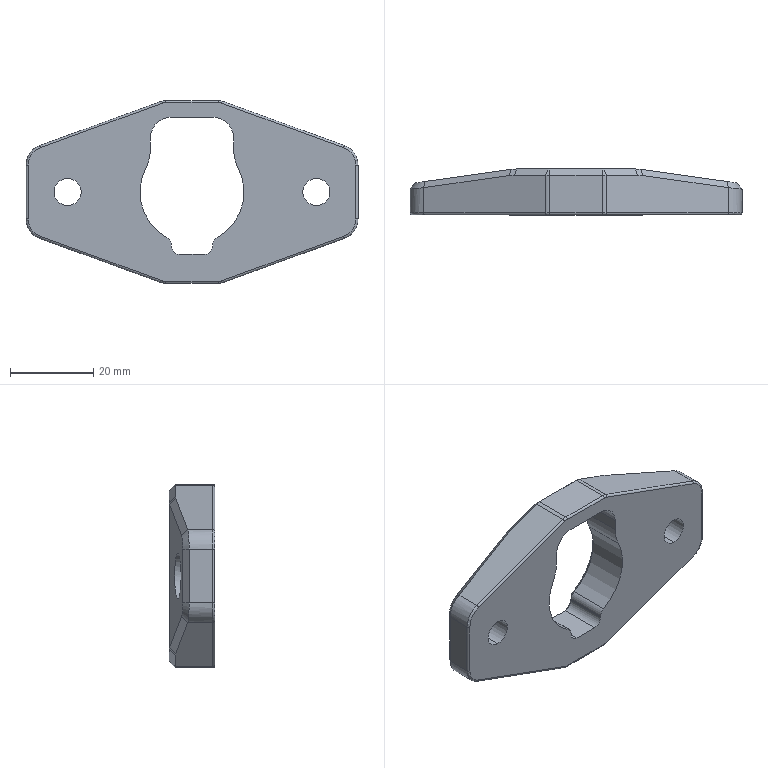Part | SolidWorks | features BaseBody 1 | 1 solid | 104 faces | box 79.834 x 11 x 44 mm | volume 19156 mm3 | plane 38 | cylinder 36 | cone 14 | spline 8 | torus 8 | commonest cylinder face diameters 1 x8 10 x6 4 x4 6 x4 6.5 x4 11 x4